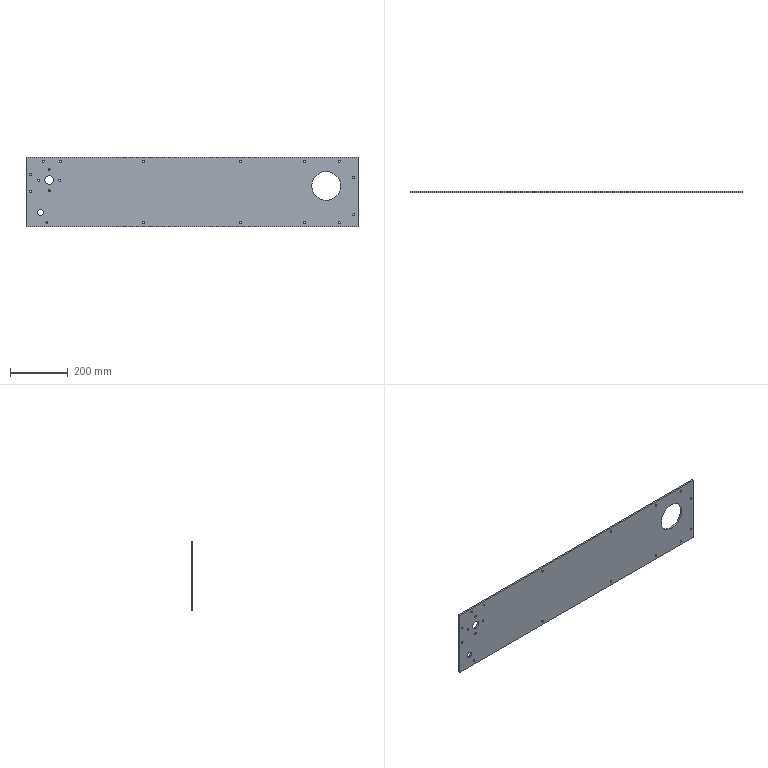Part | SolidWorks | features BaseBody 1 | 1 solid | 50 faces | box 1150 x 6 x 242 mm | volume 1612163 mm3 | cylinder 44 | plane 6 | commonest cylinder face diameters 7 x38 20 x2 30 x2 100 x2